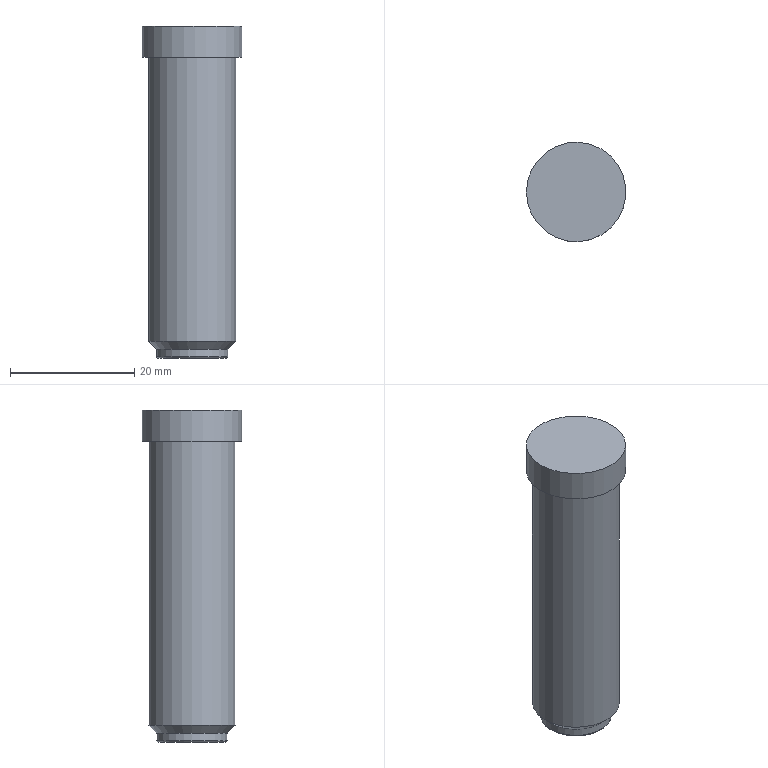Part | NX | features solid 2 | 1 solid | 8 faces | box 16 x 16 x 53.4 mm | volume 8348 mm3 | cylinder 3 | plane 3 | cone 1 | torus 1 | commonest cylinder face diameters 11.4 x1 14 x1 16 x1
STEP:
#1=CARTESIAN_POINT('',(1491.079,141.904,-30.69));
#2=VERTEX_POINT('',#1);
#3=CARTESIAN_POINT('',(1484.079,141.904,-30.69));
#4=DIRECTION('',(0.,0.,1.));
#5=DIRECTION('',(1.,0.,0.));
#6=AXIS2_PLACEMENT_3D('',#3,#4,#5);
#7=CIRCLE('',#6,7.);
#8=EDGE_CURVE('',#2,#2,#7,.T.);
#9=ORIENTED_EDGE('',*,*,#8,.T.);
#10=EDGE_LOOP('',(#9));
#11=FACE_BOUND('',#10,.T.);
#12=CARTESIAN_POINT('',(1477.079,141.904,15.));
#13=VERTEX_POINT('',#12);
#14=CARTESIAN_POINT('',(1484.079,141.904,15.));
#15=DIRECTION('',(0.,0.,-1.));
#16=DIRECTION('',(-1.,0.,0.));
#17=AXIS2_PLACEMENT_3D('',#14,#15,#16);
#18=CIRCLE('',#17,7.);
#19=EDGE_CURVE('',#13,#13,#18,.F.);
#20=ORIENTED_EDGE('',*,*,#19,.F.);
#21=EDGE_LOOP('',(#20));
#22=FACE_BOUND('',#21,.T.);
#23=CARTESIAN_POINT('',(1484.079,141.904,-33.));
#24=DIRECTION('',(0.,0.,1.));
#25=DIRECTION('',(-1.,0.,0.));
#26=AXIS2_PLACEMENT_3D('',#23,#24,#25);
#27=CYLINDRICAL_SURFACE('',#26,7.);
#28=ADVANCED_FACE('',(#11,#22),#27,.T.);
#29=CARTESIAN_POINT('',(1476.079,141.904,20.));
#30=VERTEX_POINT('',#29);
#31=CARTESIAN_POINT('',(1484.079,141.904,20.));
#32=DIRECTION('',(0.,0.,-1.));
#33=DIRECTION('',(-1.,0.,0.));
#34=AXIS2_PLACEMENT_3D('',#31,#32,#33);
#35=CIRCLE('',#34,8.);
#36=EDGE_CURVE('',#30,#30,#35,.T.);
#37=ORIENTED_EDGE('',*,*,#36,.T.);
#38=EDGE_LOOP('',(#37));
#39=FACE_BOUND('',#38,.T.);
#40=CARTESIAN_POINT('',(1476.079,141.904,15.));
#41=VERTEX_POINT('',#40);
#42=CARTESIAN_POINT('',(1484.079,141.904,15.));
#43=DIRECTION('',(0.,0.,-1.));
#44=DIRECTION('',(-1.,0.,0.));
#45=AXIS2_PLACEMENT_3D('',#42,#43,#44);
#46=CIRCLE('',#45,8.);
#47=EDGE_CURVE('',#41,#41,#46,.T.);
#48=ORIENTED_EDGE('',*,*,#47,.F.);
#49=EDGE_LOOP('',(#48));
#50=FACE_BOUND('',#49,.T.);
#51=CARTESIAN_POINT('',(1484.079,141.904,5.6));
#52=DIRECTION('',(0.,0.,-1.));
#53=DIRECTION('',(1.,0.,0.));
#54=AXIS2_PLACEMENT_3D('',#51,#52,#53);
#55=CYLINDRICAL_SURFACE('',#54,8.);
#56=ADVANCED_FACE('',(#39,#50),#55,.T.);
#57=ORIENTED_EDGE('',*,*,#19,.T.);
#58=EDGE_LOOP('',(#57));
#59=FACE_BOUND('',#58,.T.);
#60=ORIENTED_EDGE('',*,*,#47,.T.);
#61=EDGE_LOOP('',(#60));
#62=FACE_BOUND('',#61,.T.);
#63=CARTESIAN_POINT('',(1484.079,141.904,15.));
#64=DIRECTION('',(0.,0.,-1.));
#65=DIRECTION('',(1.,0.,0.));
#66=AXIS2_PLACEMENT_3D('',#63,#64,#65);
#67=PLANE('',#66);
#68=ADVANCED_FACE('',(#59,#62),#67,.T.);
#69=ORIENTED_EDGE('',*,*,#36,.F.);
#70=EDGE_LOOP('',(#69));
#71=FACE_BOUND('',#70,.T.);
#72=CARTESIAN_POINT('',(1304.995,-99.269,20.));
#73=DIRECTION('',(0.,0.,-1.));
#74=DIRECTION('',(-1.,0.,0.));
#75=AXIS2_PLACEMENT_3D('',#72,#73,#74);
#76=PLANE('',#75);
#77=ADVANCED_FACE('',(#71),#76,.F.);
#78=CARTESIAN_POINT('',(1489.779,141.904,-33.2));
#79=VERTEX_POINT('',#78);
#80=CARTESIAN_POINT('',(1484.079,141.904,-33.2));
#81=DIRECTION('',(0.,0.,1.));
#82=DIRECTION('',(1.,0.,0.));
#83=AXIS2_PLACEMENT_3D('',#80,#81,#82);
#84=CIRCLE('',#83,5.7);
#85=EDGE_CURVE('',#79,#79,#84,.T.);
#86=ORIENTED_EDGE('',*,*,#85,.T.);
#87=EDGE_LOOP('',(#86));
#88=FACE_BOUND('',#87,.T.);
#89=CARTESIAN_POINT('',(1489.779,141.904,-31.99));
#90=VERTEX_POINT('',#89);
#91=CARTESIAN_POINT('',(1484.079,141.904,-31.99));
#92=DIRECTION('',(0.,0.,1.));
#93=DIRECTION('',(1.,0.,0.));
#94=AXIS2_PLACEMENT_3D('',#91,#92,#93);
#95=CIRCLE('',#94,5.7);
#96=EDGE_CURVE('',#90,#90,#95,.F.);
#97=ORIENTED_EDGE('',*,*,#96,.T.);
#98=EDGE_LOOP('',(#97));
#99=FACE_BOUND('',#98,.T.);
#100=CARTESIAN_POINT('',(1484.079,141.904,50.75));
#101=DIRECTION('',(0.,0.,-1.));
#102=DIRECTION('',(-1.,0.,0.));
#103=AXIS2_PLACEMENT_3D('',#100,#101,#102);
#104=CYLINDRICAL_SURFACE('',#103,5.7);
#105=ADVANCED_FACE('',(#88,#99),#104,.T.);
#106=ORIENTED_EDGE('',*,*,#8,.F.);
#107=EDGE_LOOP('',(#106));
#108=FACE_BOUND('',#107,.T.);
#109=ORIENTED_EDGE('',*,*,#96,.F.);
#110=EDGE_LOOP('',(#109));
#111=FACE_BOUND('',#110,.T.);
#112=CARTESIAN_POINT('',(1484.079,141.904,-31.9));
#113=DIRECTION('',(0.,0.,1.));
#114=DIRECTION('',(1.,0.,0.));
#115=AXIS2_PLACEMENT_3D('',#112,#113,#114);
#116=CONICAL_SURFACE('',#115,5.79,0.7854);
#117=ADVANCED_FACE('',(#108,#111),#116,.T.);
#118=CARTESIAN_POINT('',(1489.579,141.904,-33.4));
#119=VERTEX_POINT('',#118);
#120=CARTESIAN_POINT('',(1484.079,141.904,-33.4));
#121=DIRECTION('',(0.,0.,1.));
#122=DIRECTION('',(1.,0.,0.));
#123=AXIS2_PLACEMENT_3D('',#120,#121,#122);
#124=CIRCLE('',#123,5.5);
#125=EDGE_CURVE('',#119,#119,#124,.F.);
#126=ORIENTED_EDGE('',*,*,#125,.T.);
#127=EDGE_LOOP('',(#126));
#128=FACE_BOUND('',#127,.T.);
#129=CARTESIAN_POINT('',(1484.079,141.904,-33.4));
#130=DIRECTION('',(0.,0.,1.));
#131=DIRECTION('',(-1.,0.,0.));
#132=AXIS2_PLACEMENT_3D('',#129,#130,#131);
#133=PLANE('',#132);
#134=ADVANCED_FACE('',(#128),#133,.F.);
#135=ORIENTED_EDGE('',*,*,#125,.F.);
#136=EDGE_LOOP('',(#135));
#137=FACE_BOUND('',#136,.T.);
#138=ORIENTED_EDGE('',*,*,#85,.F.);
#139=EDGE_LOOP('',(#138));
#140=FACE_BOUND('',#139,.T.);
#141=CARTESIAN_POINT('',(1484.079,141.904,-33.2));
#142=DIRECTION('',(0.,0.,1.));
#143=DIRECTION('',(1.,0.,0.));
#144=AXIS2_PLACEMENT_3D('',#141,#142,#143);
#145=TOROIDAL_SURFACE('',#144,5.5,0.2);
#146=ADVANCED_FACE('',(#137,#140),#145,.T.);
#147=CLOSED_SHELL('',(#28,#56,#68,#77,#105,#117,#134,#146));
#148=MANIFOLD_SOLID_BREP('',#147);
#149=(LENGTH_UNIT()NAMED_UNIT(*)SI_UNIT(.MILLI.,.METRE.));
#150=UNCERTAINTY_MEASURE_WITH_UNIT(LENGTH_MEASURE(0.00001),#149,'','');
#151=(NAMED_UNIT(*)PLANE_ANGLE_UNIT()SI_UNIT($,.RADIAN.));
#152=(NAMED_UNIT(*)SI_UNIT($,.STERADIAN.)SOLID_ANGLE_UNIT());
#153=(GEOMETRIC_REPRESENTATION_CONTEXT(3)GLOBAL_UNCERTAINTY_ASSIGNED_CONTEXT((#150))GLOBAL_UNIT_ASSIGNED_CONTEXT((#149,#151,#152))REPRESENTATION_CONTEXT('',''));
#154=ADVANCED_BREP_SHAPE_REPRESENTATION('',(#148),#153);